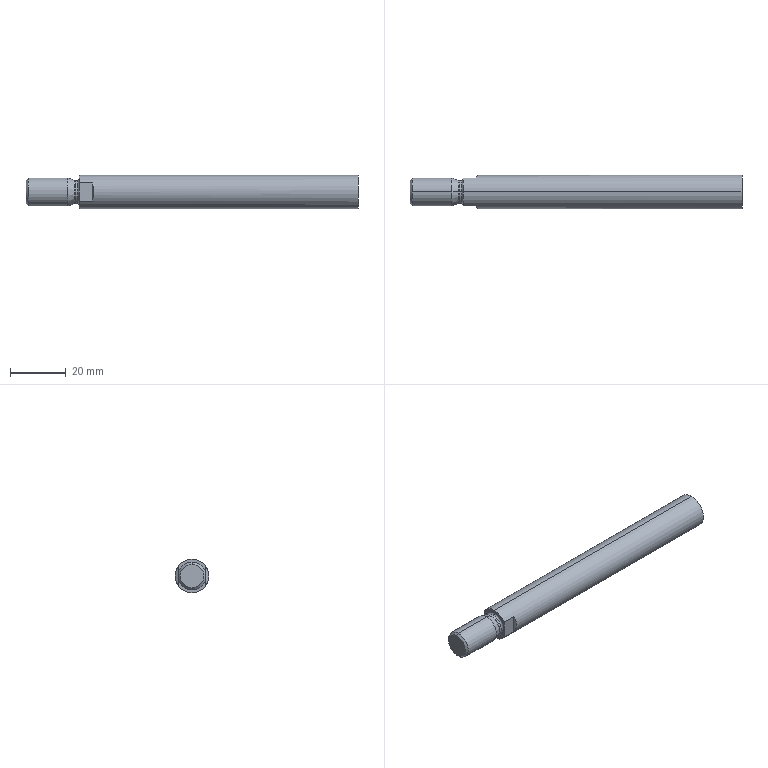Part | STEP file | Part 4 | 1 solid | 21 faces | box 119 x 12 x 12 mm | volume 12679 mm3 | plane 7 | cylinder 6 | torus 4 | cone 4 | commonest cylinder face diameters 8.2 x2 10 x2 12 x2
STEP:
#1=CARTESIAN_POINT('',(0.,0.,0.));
#2=DIRECTION('',(0.,0.,1.));
#3=DIRECTION('',(1.,0.,0.));
#4=AXIS2_PLACEMENT_3D('',#1,#2,#3);
#5=CARTESIAN_POINT('',(-7.699,0.,4.136));
#6=VERTEX_POINT('',#5);
#7=CARTESIAN_POINT('',(-7.494,0.,4.1));
#8=VERTEX_POINT('',#7);
#9=CARTESIAN_POINT('',(-7.494,0.,4.7));
#10=DIRECTION('',(0.,-1.,0.));
#11=DIRECTION('',(0.,0.,-1.));
#12=AXIS2_PLACEMENT_3D('',#9,#10,#11);
#13=CIRCLE('',#12,0.6);
#14=CARTESIAN_POINT('',(-7.494,0.,0.));
#15=DIRECTION('',(-1.,0.,0.));
#16=DIRECTION('',(0.,0.,1.));
#17=AXIS2_PLACEMENT_3D('',#14,#15,#16);
#18=TOROIDAL_SURFACE('',#17,4.7,0.6);
#19=CARTESIAN_POINT('',(6.283,-3.142));
#20=DIRECTION('',(0.,1.));
#21=VECTOR('',#20,1.);
#22=LINE('',#19,#21);
#23=(GEOMETRIC_REPRESENTATION_CONTEXT(2)PARAMETRIC_REPRESENTATION_CONTEXT()REPRESENTATION_CONTEXT('',''));
#24=DEFINITIONAL_REPRESENTATION('',(#22),#23);
#25=PCURVE('',#18,#24);
#26=CARTESIAN_POINT('',(-7.494,0.,0.));
#27=DIRECTION('',(-1.,0.,0.));
#28=DIRECTION('',(0.,0.,1.));
#29=AXIS2_PLACEMENT_3D('',#26,#27,#28);
#30=TOROIDAL_SURFACE('',#29,4.7,0.6);
#31=CARTESIAN_POINT('',(0.,-3.142));
#32=DIRECTION('',(0.,1.));
#33=VECTOR('',#32,1.);
#34=LINE('',#31,#33);
#35=(GEOMETRIC_REPRESENTATION_CONTEXT(2)PARAMETRIC_REPRESENTATION_CONTEXT()REPRESENTATION_CONTEXT('',''));
#36=DEFINITIONAL_REPRESENTATION('',(#34),#35);
#37=PCURVE('',#30,#36);
#38=SURFACE_CURVE('',#13,(#25,#37),.PCURVE_S1.);
#39=EDGE_CURVE('',#6,#8,#38,.T.);
#40=ORIENTED_EDGE('',*,*,#39,.T.);
#41=CARTESIAN_POINT('',(-7.494,0.,-4.1));
#42=VERTEX_POINT('',#41);
#43=CARTESIAN_POINT('',(-7.494,0.,0.));
#44=DIRECTION('',(1.,0.,0.));
#45=DIRECTION('',(0.,0.,1.));
#46=AXIS2_PLACEMENT_3D('',#43,#44,#45);
#47=CIRCLE('',#46,4.1);
#48=CARTESIAN_POINT('',(6.283,3.142));
#49=DIRECTION('',(-1.,0.));
#50=VECTOR('',#49,1.);
#51=LINE('',#48,#50);
#52=(GEOMETRIC_REPRESENTATION_CONTEXT(2)PARAMETRIC_REPRESENTATION_CONTEXT()REPRESENTATION_CONTEXT('',''));
#53=DEFINITIONAL_REPRESENTATION('',(#51),#52);
#54=PCURVE('',#18,#53);
#55=CARTESIAN_POINT('',(-7.6,0.,0.));
#56=DIRECTION('',(1.,0.,0.));
#57=DIRECTION('',(0.,0.,-1.));
#58=AXIS2_PLACEMENT_3D('',#55,#56,#57);
#59=CYLINDRICAL_SURFACE('',#58,4.1);
#60=CARTESIAN_POINT('',(3.142,0.1058));
#61=DIRECTION('',(1.,0.));
#62=VECTOR('',#61,1.);
#63=LINE('',#60,#62);
#64=(GEOMETRIC_REPRESENTATION_CONTEXT(2)PARAMETRIC_REPRESENTATION_CONTEXT()REPRESENTATION_CONTEXT('',''));
#65=DEFINITIONAL_REPRESENTATION('',(#63),#64);
#66=PCURVE('',#59,#65);
#67=SURFACE_CURVE('',#47,(#54,#66),.PCURVE_S1.);
#68=EDGE_CURVE('',#8,#42,#67,.T.);
#69=ORIENTED_EDGE('',*,*,#68,.T.);
#70=CARTESIAN_POINT('',(-7.699,0.,-4.136));
#71=VERTEX_POINT('',#70);
#72=CARTESIAN_POINT('',(-7.494,0.,-4.7));
#73=DIRECTION('',(0.,1.,0.));
#74=DIRECTION('',(0.,0.,1.));
#75=AXIS2_PLACEMENT_3D('',#72,#73,#74);
#76=CIRCLE('',#75,0.6);
#77=CARTESIAN_POINT('',(3.142,-3.142));
#78=DIRECTION('',(0.,1.));
#79=VECTOR('',#78,1.);
#80=LINE('',#77,#79);
#81=(GEOMETRIC_REPRESENTATION_CONTEXT(2)PARAMETRIC_REPRESENTATION_CONTEXT()REPRESENTATION_CONTEXT('',''));
#82=DEFINITIONAL_REPRESENTATION('',(#80),#81);
#83=PCURVE('',#18,#82);
#84=CARTESIAN_POINT('',(3.142,-3.142));
#85=DIRECTION('',(0.,1.));
#86=VECTOR('',#85,1.);
#87=LINE('',#84,#86);
#88=(GEOMETRIC_REPRESENTATION_CONTEXT(2)PARAMETRIC_REPRESENTATION_CONTEXT()REPRESENTATION_CONTEXT('',''));
#89=DEFINITIONAL_REPRESENTATION('',(#87),#88);
#90=PCURVE('',#30,#89);
#91=SURFACE_CURVE('',#76,(#83,#90),.PCURVE_S1.);
#92=EDGE_CURVE('',#71,#42,#91,.T.);
#93=ORIENTED_EDGE('',*,*,#92,.F.);
#94=CARTESIAN_POINT('',(-7.699,0.,0.));
#95=DIRECTION('',(-1.,0.,0.));
#96=DIRECTION('',(0.,0.,1.));
#97=AXIS2_PLACEMENT_3D('',#94,#95,#96);
#98=CIRCLE('',#97,4.136);
#99=CARTESIAN_POINT('',(0.,2.793));
#100=DIRECTION('',(1.,0.));
#101=VECTOR('',#100,1.);
#102=LINE('',#99,#101);
#103=(GEOMETRIC_REPRESENTATION_CONTEXT(2)PARAMETRIC_REPRESENTATION_CONTEXT()REPRESENTATION_CONTEXT('',''));
#104=DEFINITIONAL_REPRESENTATION('',(#102),#103);
#105=PCURVE('',#18,#104);
#106=CARTESIAN_POINT('',(-7.6,0.,0.));
#107=DIRECTION('',(-1.,0.,0.));
#108=DIRECTION('',(0.,0.,1.));
#109=AXIS2_PLACEMENT_3D('',#106,#107,#108);
#110=CONICAL_SURFACE('',#109,4.1,0.3491);
#111=CARTESIAN_POINT('',(0.,0.09942));
#112=DIRECTION('',(1.,0.));
#113=VECTOR('',#112,1.);
#114=LINE('',#111,#113);
#115=(GEOMETRIC_REPRESENTATION_CONTEXT(2)PARAMETRIC_REPRESENTATION_CONTEXT()REPRESENTATION_CONTEXT('',''));
#116=DEFINITIONAL_REPRESENTATION('',(#114),#115);
#117=PCURVE('',#110,#116);
#118=SURFACE_CURVE('',#98,(#105,#117),.PCURVE_S1.);
#119=EDGE_CURVE('',#71,#6,#118,.T.);
#120=ORIENTED_EDGE('',*,*,#119,.T.);
#121=EDGE_LOOP('',(#40,#69,#93,#120));
#122=FACE_BOUND('',#121,.F.);
#123=ADVANCED_FACE('',(#122),#18,.F.);
#124=CARTESIAN_POINT('',(-6.7,0.,4.1));
#125=VERTEX_POINT('',#124);
#126=CARTESIAN_POINT('',(-6.1,0.,4.7));
#127=VERTEX_POINT('',#126);
#128=CARTESIAN_POINT('',(-6.7,0.,4.7));
#129=DIRECTION('',(0.,-1.,0.));
#130=DIRECTION('',(0.,0.,-1.));
#131=AXIS2_PLACEMENT_3D('',#128,#129,#130);
#132=CIRCLE('',#131,0.6);
#133=CARTESIAN_POINT('',(-6.7,0.,0.));
#134=DIRECTION('',(-1.,0.,0.));
#135=DIRECTION('',(0.,0.,1.));
#136=AXIS2_PLACEMENT_3D('',#133,#134,#135);
#137=TOROIDAL_SURFACE('',#136,4.7,0.6);
#138=CARTESIAN_POINT('',(6.283,3.142));
#139=DIRECTION('',(0.,1.));
#140=VECTOR('',#139,1.);
#141=LINE('',#138,#140);
#142=(GEOMETRIC_REPRESENTATION_CONTEXT(2)PARAMETRIC_REPRESENTATION_CONTEXT()REPRESENTATION_CONTEXT('',''));
#143=DEFINITIONAL_REPRESENTATION('',(#141),#142);
#144=PCURVE('',#137,#143);
#145=CARTESIAN_POINT('',(-6.7,0.,0.));
#146=DIRECTION('',(-1.,0.,0.));
#147=DIRECTION('',(0.,0.,1.));
#148=AXIS2_PLACEMENT_3D('',#145,#146,#147);
#149=TOROIDAL_SURFACE('',#148,4.7,0.6);
#150=CARTESIAN_POINT('',(0.,3.142));
#151=DIRECTION('',(0.,1.));
#152=VECTOR('',#151,1.);
#153=LINE('',#150,#152);
#154=(GEOMETRIC_REPRESENTATION_CONTEXT(2)PARAMETRIC_REPRESENTATION_CONTEXT()REPRESENTATION_CONTEXT('',''));
#155=DEFINITIONAL_REPRESENTATION('',(#153),#154);
#156=PCURVE('',#149,#155);
#157=SURFACE_CURVE('',#132,(#144,#156),.PCURVE_S1.);
#158=EDGE_CURVE('',#125,#127,#157,.T.);
#159=ORIENTED_EDGE('',*,*,#158,.T.);
#160=CARTESIAN_POINT('',(-6.1,0.,-4.7));
#161=VERTEX_POINT('',#160);
#162=CARTESIAN_POINT('',(-6.1,0.,0.));
#163=DIRECTION('',(1.,0.,0.));
#164=DIRECTION('',(0.,0.,1.));
#165=AXIS2_PLACEMENT_3D('',#162,#163,#164);
#166=CIRCLE('',#165,4.7);
#167=CARTESIAN_POINT('',(6.283,4.712));
#168=DIRECTION('',(-1.,0.));
#169=VECTOR('',#168,1.);
#170=LINE('',#167,#169);
#171=(GEOMETRIC_REPRESENTATION_CONTEXT(2)PARAMETRIC_REPRESENTATION_CONTEXT()REPRESENTATION_CONTEXT('',''));
#172=DEFINITIONAL_REPRESENTATION('',(#170),#171);
#173=PCURVE('',#137,#172);
#174=CARTESIAN_POINT('',(-6.1,6.,0.));
#175=DIRECTION('',(-1.,0.,0.));
#176=DIRECTION('',(0.,0.,1.));
#177=AXIS2_PLACEMENT_3D('',#174,#175,#176);
#178=PLANE('',#177);
#179=CARTESIAN_POINT('',(4.7,-6.));
#180=CARTESIAN_POINT('',(4.7,-14.141));
#181=CARTESIAN_POINT('',(-2.35,-10.07));
#182=CARTESIAN_POINT('',(-9.4,-6.));
#183=CARTESIAN_POINT('',(-2.35,-1.93));
#184=CARTESIAN_POINT('',(4.7,2.141));
#185=CARTESIAN_POINT('',(4.7,-6.));
#186=(BOUNDED_CURVE()B_SPLINE_CURVE(2,(#179,#180,#181,#182,#183,#184,#185),.UNSPECIFIED.,.T.,.F.)B_SPLINE_CURVE_WITH_KNOTS((1,2,2,2,2,1),(-2.094,0.,2.094,4.189,6.283,8.378),.UNSPECIFIED.)CURVE()GEOMETRIC_REPRESENTATION_ITEM()RATIONAL_B_SPLINE_CURVE((1.,0.5,1.,0.5,1.,0.5,1.))REPRESENTATION_ITEM(''));
#187=(GEOMETRIC_REPRESENTATION_CONTEXT(2)PARAMETRIC_REPRESENTATION_CONTEXT()REPRESENTATION_CONTEXT('',''));
#188=DEFINITIONAL_REPRESENTATION('',(#186),#187);
#189=PCURVE('',#178,#188);
#190=SURFACE_CURVE('',#166,(#173,#189),.PCURVE_S1.);
#191=EDGE_CURVE('',#127,#161,#190,.T.);
#192=ORIENTED_EDGE('',*,*,#191,.T.);
#193=CARTESIAN_POINT('',(-6.7,0.,-4.1));
#194=VERTEX_POINT('',#193);
#195=CARTESIAN_POINT('',(-6.7,0.,-4.7));
#196=DIRECTION('',(0.,1.,0.));
#197=DIRECTION('',(0.,0.,1.));
#198=AXIS2_PLACEMENT_3D('',#195,#196,#197);
#199=CIRCLE('',#198,0.6);
#200=CARTESIAN_POINT('',(3.142,3.142));
#201=DIRECTION('',(0.,1.));
#202=VECTOR('',#201,1.);
#203=LINE('',#200,#202);
#204=(GEOMETRIC_REPRESENTATION_CONTEXT(2)PARAMETRIC_REPRESENTATION_CONTEXT()REPRESENTATION_CONTEXT('',''));
#205=DEFINITIONAL_REPRESENTATION('',(#203),#204);
#206=PCURVE('',#137,#205);
#207=CARTESIAN_POINT('',(3.142,3.142));
#208=DIRECTION('',(0.,1.));
#209=VECTOR('',#208,1.);
#210=LINE('',#207,#209);
#211=(GEOMETRIC_REPRESENTATION_CONTEXT(2)PARAMETRIC_REPRESENTATION_CONTEXT()REPRESENTATION_CONTEXT('',''));
#212=DEFINITIONAL_REPRESENTATION('',(#210),#211);
#213=PCURVE('',#149,#212);
#214=SURFACE_CURVE('',#199,(#206,#213),.PCURVE_S1.);
#215=EDGE_CURVE('',#194,#161,#214,.T.);
#216=ORIENTED_EDGE('',*,*,#215,.F.);
#217=CARTESIAN_POINT('',(-6.7,0.,0.));
#218=DIRECTION('',(-1.,0.,0.));
#219=DIRECTION('',(0.,0.,1.));
#220=AXIS2_PLACEMENT_3D('',#217,#218,#219);
#221=CIRCLE('',#220,4.1);
#222=CARTESIAN_POINT('',(0.,3.142));
#223=DIRECTION('',(1.,0.));
#224=VECTOR('',#223,1.);
#225=LINE('',#222,#224);
#226=(GEOMETRIC_REPRESENTATION_CONTEXT(2)PARAMETRIC_REPRESENTATION_CONTEXT()REPRESENTATION_CONTEXT('',''));
#227=DEFINITIONAL_REPRESENTATION('',(#225),#226);
#228=PCURVE('',#137,#227);
#229=CARTESIAN_POINT('',(9.425,0.9));
#230=DIRECTION('',(-1.,0.));
#231=VECTOR('',#230,1.);
#232=LINE('',#229,#231);
#233=(GEOMETRIC_REPRESENTATION_CONTEXT(2)PARAMETRIC_REPRESENTATION_CONTEXT()REPRESENTATION_CONTEXT('',''));
#234=DEFINITIONAL_REPRESENTATION('',(#232),#233);
#235=PCURVE('',#59,#234);
#236=SURFACE_CURVE('',#221,(#228,#235),.PCURVE_S1.);
#237=EDGE_CURVE('',#194,#125,#236,.T.);
#238=ORIENTED_EDGE('',*,*,#237,.T.);
#239=EDGE_LOOP('',(#159,#192,#216,#238));
#240=FACE_BOUND('',#239,.F.);
#241=ADVANCED_FACE('',(#240),#137,.F.);
#242=CARTESIAN_POINT('',(-25.1,0.,4.233));
#243=VERTEX_POINT('',#242);
#244=CARTESIAN_POINT('',(-25.1,0.,-4.233));
#245=VERTEX_POINT('',#244);
#246=CARTESIAN_POINT('',(-25.1,0.,0.));
#247=DIRECTION('',(-1.,0.,0.));
#248=DIRECTION('',(0.,0.,1.));
#249=AXIS2_PLACEMENT_3D('',#246,#247,#248);
#250=CIRCLE('',#249,4.233);
#251=CARTESIAN_POINT('',(-25.1,0.,0.));
#252=DIRECTION('',(1.,0.,0.));
#253=DIRECTION('',(0.,0.,-1.));
#254=AXIS2_PLACEMENT_3D('',#251,#252,#253);
#255=CONICAL_SURFACE('',#254,4.233,0.7854);
#256=CARTESIAN_POINT('',(3.142,0.));
#257=DIRECTION('',(-1.,0.));
#258=VECTOR('',#257,1.);
#259=LINE('',#256,#258);
#260=(GEOMETRIC_REPRESENTATION_CONTEXT(2)PARAMETRIC_REPRESENTATION_CONTEXT()REPRESENTATION_CONTEXT('',''));
#261=DEFINITIONAL_REPRESENTATION('',(#259),#260);
#262=PCURVE('',#255,#261);
#263=CARTESIAN_POINT('',(-25.1,0.,0.));
#264=DIRECTION('',(-1.,0.,0.));
#265=DIRECTION('',(0.,0.,1.));
#266=AXIS2_PLACEMENT_3D('',#263,#264,#265);
#267=PLANE('',#266);
#268=CARTESIAN_POINT('',(0.,0.));
#269=DIRECTION('',(1.,0.));
#270=AXIS2_PLACEMENT_2D('',#268,#269);
#271=CIRCLE('',#270,4.233);
#272=(GEOMETRIC_REPRESENTATION_CONTEXT(2)PARAMETRIC_REPRESENTATION_CONTEXT()REPRESENTATION_CONTEXT('',''));
#273=DEFINITIONAL_REPRESENTATION('',(#271),#272);
#274=PCURVE('',#267,#273);
#275=SURFACE_CURVE('',#250,(#262,#274),.PCURVE_S1.);
#276=EDGE_CURVE('',#243,#245,#275,.T.);
#277=ORIENTED_EDGE('',*,*,#276,.F.);
#278=CARTESIAN_POINT('',(-24.333,0.,5.));
#279=VERTEX_POINT('',#278);
#280=CARTESIAN_POINT('',(-25.1,0.,4.233));
#281=DIRECTION('',(0.7071,0.,0.7071));
#282=VECTOR('',#281,1.);
#283=LINE('',#280,#282);
#284=CARTESIAN_POINT('',(3.142,0.));
#285=DIRECTION('',(0.,1.));
#286=VECTOR('',#285,1.);
#287=LINE('',#284,#286);
#288=(GEOMETRIC_REPRESENTATION_CONTEXT(2)PARAMETRIC_REPRESENTATION_CONTEXT()REPRESENTATION_CONTEXT('',''));
#289=DEFINITIONAL_REPRESENTATION('',(#287),#288);
#290=PCURVE('',#255,#289);
#291=CARTESIAN_POINT('',(-25.1,0.,0.));
#292=DIRECTION('',(1.,0.,0.));
#293=DIRECTION('',(0.,0.,-1.));
#294=AXIS2_PLACEMENT_3D('',#291,#292,#293);
#295=CONICAL_SURFACE('',#294,4.233,0.7854);
#296=CARTESIAN_POINT('',(3.142,0.));
#297=DIRECTION('',(0.,1.));
#298=VECTOR('',#297,1.);
#299=LINE('',#296,#298);
#300=(GEOMETRIC_REPRESENTATION_CONTEXT(2)PARAMETRIC_REPRESENTATION_CONTEXT()REPRESENTATION_CONTEXT('',''));
#301=DEFINITIONAL_REPRESENTATION('',(#299),#300);
#302=PCURVE('',#295,#301);
#303=SURFACE_CURVE('',#283,(#290,#302),.PCURVE_S1.);
#304=EDGE_CURVE('',#243,#279,#303,.T.);
#305=ORIENTED_EDGE('',*,*,#304,.T.);
#306=CARTESIAN_POINT('',(-24.333,0.,-5.));
#307=VERTEX_POINT('',#306);
#308=CARTESIAN_POINT('',(-24.333,0.,0.));
#309=DIRECTION('',(1.,0.,0.));
#310=DIRECTION('',(0.,0.,1.));
#311=AXIS2_PLACEMENT_3D('',#308,#309,#310);
#312=CIRCLE('',#311,5.);
#313=CARTESIAN_POINT('',(-3.142,0.767));
#314=DIRECTION('',(1.,0.));
#315=VECTOR('',#314,1.);
#316=LINE('',#313,#315);
#317=(GEOMETRIC_REPRESENTATION_CONTEXT(2)PARAMETRIC_REPRESENTATION_CONTEXT()REPRESENTATION_CONTEXT('',''));
#318=DEFINITIONAL_REPRESENTATION('',(#316),#317);
#319=PCURVE('',#255,#318);
#320=CARTESIAN_POINT('',(-25.1,0.,0.));
#321=DIRECTION('',(1.,0.,0.));
#322=DIRECTION('',(0.,0.,-1.));
#323=AXIS2_PLACEMENT_3D('',#320,#321,#322);
#324=CYLINDRICAL_SURFACE('',#323,5.);
#325=CARTESIAN_POINT('',(-3.142,0.767));
#326=DIRECTION('',(1.,0.));
#327=VECTOR('',#326,1.);
#328=LINE('',#325,#327);
#329=(GEOMETRIC_REPRESENTATION_CONTEXT(2)PARAMETRIC_REPRESENTATION_CONTEXT()REPRESENTATION_CONTEXT('',''));
#330=DEFINITIONAL_REPRESENTATION('',(#328),#329);
#331=PCURVE('',#324,#330);
#332=SURFACE_CURVE('',#312,(#319,#331),.PCURVE_S1.);
#333=EDGE_CURVE('',#307,#279,#332,.T.);
#334=ORIENTED_EDGE('',*,*,#333,.F.);
#335=CARTESIAN_POINT('',(-25.1,0.,-4.233));
#336=DIRECTION('',(0.7071,0.,-0.7071));
#337=VECTOR('',#336,1.);
#338=LINE('',#335,#337);
#339=CARTESIAN_POINT('',(0.,0.));
#340=DIRECTION('',(0.,1.));
#341=VECTOR('',#340,1.);
#342=LINE('',#339,#341);
#343=(GEOMETRIC_REPRESENTATION_CONTEXT(2)PARAMETRIC_REPRESENTATION_CONTEXT()REPRESENTATION_CONTEXT('',''));
#344=DEFINITIONAL_REPRESENTATION('',(#342),#343);
#345=PCURVE('',#255,#344);
#346=CARTESIAN_POINT('',(6.283,0.));
#347=DIRECTION('',(0.,1.));
#348=VECTOR('',#347,1.);
#349=LINE('',#346,#348);
#350=(GEOMETRIC_REPRESENTATION_CONTEXT(2)PARAMETRIC_REPRESENTATION_CONTEXT()REPRESENTATION_CONTEXT('',''));
#351=DEFINITIONAL_REPRESENTATION('',(#349),#350);
#352=PCURVE('',#295,#351);
#353=SURFACE_CURVE('',#338,(#345,#352),.PCURVE_S1.);
#354=EDGE_CURVE('',#245,#307,#353,.T.);
#355=ORIENTED_EDGE('',*,*,#354,.F.);
#356=EDGE_LOOP('',(#277,#305,#334,#355));
#357=FACE_BOUND('',#356,.T.);
#358=ADVANCED_FACE('',(#357),#255,.T.);
#359=ORIENTED_EDGE('',*,*,#333,.T.);
#360=CARTESIAN_POINT('',(-10.073,0.,5.));
#361=VERTEX_POINT('',#360);
#362=CARTESIAN_POINT('',(-25.1,0.,5.));
#363=DIRECTION('',(1.,0.,0.));
#364=VECTOR('',#363,1.);
#365=LINE('',#362,#364);
#366=CARTESIAN_POINT('',(3.142,0.));
#367=DIRECTION('',(0.,1.));
#368=VECTOR('',#367,1.);
#369=LINE('',#366,#368);
#370=(GEOMETRIC_REPRESENTATION_CONTEXT(2)PARAMETRIC_REPRESENTATION_CONTEXT()REPRESENTATION_CONTEXT('',''));
#371=DEFINITIONAL_REPRESENTATION('',(#369),#370);
#372=PCURVE('',#324,#371);
#373=CARTESIAN_POINT('',(-25.1,0.,0.));
#374=DIRECTION('',(1.,0.,0.));
#375=DIRECTION('',(0.,0.,-1.));
#376=AXIS2_PLACEMENT_3D('',#373,#374,#375);
#377=CYLINDRICAL_SURFACE('',#376,5.);
#378=CARTESIAN_POINT('',(3.142,0.));
#379=DIRECTION('',(0.,1.));
#380=VECTOR('',#379,1.);
#381=LINE('',#378,#380);
#382=(GEOMETRIC_REPRESENTATION_CONTEXT(2)PARAMETRIC_REPRESENTATION_CONTEXT()REPRESENTATION_CONTEXT('',''));
#383=DEFINITIONAL_REPRESENTATION('',(#381),#382);
#384=PCURVE('',#377,#383);
#385=SURFACE_CURVE('',#365,(#372,#384),.PCURVE_S1.);
#386=EDGE_CURVE('',#279,#361,#385,.T.);
#387=ORIENTED_EDGE('',*,*,#386,.T.);
#388=CARTESIAN_POINT('',(-10.073,0.,-5.));
#389=VERTEX_POINT('',#388);
#390=CARTESIAN_POINT('',(-10.073,0.,0.));
#391=DIRECTION('',(-1.,0.,0.));
#392=DIRECTION('',(0.,0.,1.));
#393=AXIS2_PLACEMENT_3D('',#390,#391,#392);
#394=CIRCLE('',#393,5.);
#395=CARTESIAN_POINT('',(3.142,15.027));
#396=DIRECTION('',(-1.,0.));
#397=VECTOR('',#396,1.);
#398=LINE('',#395,#397);
#399=(GEOMETRIC_REPRESENTATION_CONTEXT(2)PARAMETRIC_REPRESENTATION_CONTEXT()REPRESENTATION_CONTEXT('',''));
#400=DEFINITIONAL_REPRESENTATION('',(#398),#399);
#401=PCURVE('',#324,#400);
#402=CARTESIAN_POINT('',(-7.6,0.,0.));
#403=DIRECTION('',(-1.,0.,0.));
#404=DIRECTION('',(0.,0.,1.));
#405=AXIS2_PLACEMENT_3D('',#402,#403,#404);
#406=CONICAL_SURFACE('',#405,4.1,0.3491);
#407=CARTESIAN_POINT('',(0.,2.473));
#408=DIRECTION('',(1.,0.));
#409=VECTOR('',#408,1.);
#410=LINE('',#407,#409);
#411=(GEOMETRIC_REPRESENTATION_CONTEXT(2)PARAMETRIC_REPRESENTATION_CONTEXT()REPRESENTATION_CONTEXT('',''));
#412=DEFINITIONAL_REPRESENTATION('',(#410),#411);
#413=PCURVE('',#406,#412);
#414=SURFACE_CURVE('',#394,(#401,#413),.PCURVE_S1.);
#415=EDGE_CURVE('',#361,#389,#414,.T.);
#416=ORIENTED_EDGE('',*,*,#415,.T.);
#417=CARTESIAN_POINT('',(-25.1,0.,-5.));
#418=DIRECTION('',(1.,0.,0.));
#419=VECTOR('',#418,1.);
#420=LINE('',#417,#419);
#421=CARTESIAN_POINT('',(0.,0.));
#422=DIRECTION('',(0.,1.));
#423=VECTOR('',#422,1.);
#424=LINE('',#421,#423);
#425=(GEOMETRIC_REPRESENTATION_CONTEXT(2)PARAMETRIC_REPRESENTATION_CONTEXT()REPRESENTATION_CONTEXT('',''));
#426=DEFINITIONAL_REPRESENTATION('',(#424),#425);
#427=PCURVE('',#324,#426);
#428=CARTESIAN_POINT('',(6.283,0.));
#429=DIRECTION('',(0.,1.));
#430=VECTOR('',#429,1.);
#431=LINE('',#428,#430);
#432=(GEOMETRIC_REPRESENTATION_CONTEXT(2)PARAMETRIC_REPRESENTATION_CONTEXT()REPRESENTATION_CONTEXT('',''));
#433=DEFINITIONAL_REPRESENTATION('',(#431),#432);
#434=PCURVE('',#377,#433);
#435=SURFACE_CURVE('',#420,(#427,#434),.PCURVE_S1.);
#436=EDGE_CURVE('',#307,#389,#435,.T.);
#437=ORIENTED_EDGE('',*,*,#436,.F.);
#438=EDGE_LOOP('',(#359,#387,#416,#437));
#439=FACE_BOUND('',#438,.T.);
#440=ADVANCED_FACE('',(#439),#324,.T.);
#441=CARTESIAN_POINT('',(-7.699,0.,0.));
#442=DIRECTION('',(-1.,0.,0.));
#443=DIRECTION('',(0.,0.,1.));
#444=AXIS2_PLACEMENT_3D('',#441,#442,#443);
#445=CIRCLE('',#444,4.136);
#446=CARTESIAN_POINT('',(0.,0.09942));
#447=DIRECTION('',(1.,0.));
#448=VECTOR('',#447,1.);
#449=LINE('',#446,#448);
#450=(GEOMETRIC_REPRESENTATION_CONTEXT(2)PARAMETRIC_REPRESENTATION_CONTEXT()REPRESENTATION_CONTEXT('',''));
#451=DEFINITIONAL_REPRESENTATION('',(#449),#450);
#452=PCURVE('',#406,#451);
#453=CARTESIAN_POINT('',(0.,2.793));
#454=DIRECTION('',(1.,0.));
#455=VECTOR('',#454,1.);
#456=LINE('',#453,#455);
#457=(GEOMETRIC_REPRESENTATION_CONTEXT(2)PARAMETRIC_REPRESENTATION_CONTEXT()REPRESENTATION_CONTEXT('',''));
#458=DEFINITIONAL_REPRESENTATION('',(#456),#457);
#459=PCURVE('',#30,#458);
#460=SURFACE_CURVE('',#445,(#452,#459),.PCURVE_S1.);
#461=EDGE_CURVE('',#6,#71,#460,.T.);
#462=ORIENTED_EDGE('',*,*,#461,.T.);
#463=CARTESIAN_POINT('',(-7.6,0.,-4.1));
#464=DIRECTION('',(-0.9397,0.,-0.342));
#465=VECTOR('',#464,1.);
#466=LINE('',#463,#465);
#467=CARTESIAN_POINT('',(3.142,0.));
#468=DIRECTION('',(0.,1.));
#469=VECTOR('',#468,1.);
#470=LINE('',#467,#469);
#471=(GEOMETRIC_REPRESENTATION_CONTEXT(2)PARAMETRIC_REPRESENTATION_CONTEXT()REPRESENTATION_CONTEXT('',''));
#472=DEFINITIONAL_REPRESENTATION('',(#470),#471);
#473=PCURVE('',#406,#472);
#474=CARTESIAN_POINT('',(3.142,0.));
#475=DIRECTION('',(0.,1.));
#476=VECTOR('',#475,1.);
#477=LINE('',#474,#476);
#478=(GEOMETRIC_REPRESENTATION_CONTEXT(2)PARAMETRIC_REPRESENTATION_CONTEXT()REPRESENTATION_CONTEXT('',''));
#479=DEFINITIONAL_REPRESENTATION('',(#477),#478);
#480=PCURVE('',#110,#479);
#481=SURFACE_CURVE('',#466,(#473,#480),.PCURVE_S1.);
#482=EDGE_CURVE('',#71,#389,#481,.T.);
#483=ORIENTED_EDGE('',*,*,#482,.T.);
#484=ORIENTED_EDGE('',*,*,#415,.F.);
#485=CARTESIAN_POINT('',(-7.6,0.,4.1));
#486=DIRECTION('',(-0.9397,0.,0.342));
#487=VECTOR('',#486,1.);
#488=LINE('',#485,#487);
#489=CARTESIAN_POINT('',(0.,0.));
#490=DIRECTION('',(0.,1.));
#491=VECTOR('',#490,1.);
#492=LINE('',#489,#491);
#493=(GEOMETRIC_REPRESENTATION_CONTEXT(2)PARAMETRIC_REPRESENTATION_CONTEXT()REPRESENTATION_CONTEXT('',''));
#494=DEFINITIONAL_REPRESENTATION('',(#492),#493);
#495=PCURVE('',#406,#494);
#496=CARTESIAN_POINT('',(6.283,0.));
#497=DIRECTION('',(0.,1.));
#498=VECTOR('',#497,1.);
#499=LINE('',#496,#498);
#500=(GEOMETRIC_REPRESENTATION_CONTEXT(2)PARAMETRIC_REPRESENTATION_CONTEXT()REPRESENTATION_CONTEXT('',''));
#501=DEFINITIONAL_REPRESENTATION('',(#499),#500);
#502=PCURVE('',#110,#501);
#503=SURFACE_CURVE('',#488,(#495,#502),.PCURVE_S1.);
#504=EDGE_CURVE('',#6,#361,#503,.T.);
#505=ORIENTED_EDGE('',*,*,#504,.F.);
#506=EDGE_LOOP('',(#462,#483,#484,#505));
#507=FACE_BOUND('',#506,.T.);
#508=ADVANCED_FACE('',(#507),#406,.T.);
#509=CARTESIAN_POINT('',(-7.494,0.,0.));
#510=DIRECTION('',(1.,0.,0.));
#511=DIRECTION('',(0.,0.,1.));
#512=AXIS2_PLACEMENT_3D('',#509,#510,#511);
#513=CIRCLE('',#512,4.1);
#514=CARTESIAN_POINT('',(-7.6,0.,0.));
#515=DIRECTION('',(1.,0.,0.));
#516=DIRECTION('',(0.,0.,-1.));
#517=AXIS2_PLACEMENT_3D('',#514,#515,#516);
#518=CYLINDRICAL_SURFACE('',#517,4.1);
#519=CARTESIAN_POINT('',(-3.142,0.1058));
#520=DIRECTION('',(1.,0.));
#521=VECTOR('',#520,1.);
#522=LINE('',#519,#521);
#523=(GEOMETRIC_REPRESENTATION_CONTEXT(2)PARAMETRIC_REPRESENTATION_CONTEXT()REPRESENTATION_CONTEXT('',''));
#524=DEFINITIONAL_REPRESENTATION('',(#522),#523);
#525=PCURVE('',#518,#524);
#526=CARTESIAN_POINT('',(6.283,3.142));
#527=DIRECTION('',(-1.,0.));
#528=VECTOR('',#527,1.);
#529=LINE('',#526,#528);
#530=(GEOMETRIC_REPRESENTATION_CONTEXT(2)PARAMETRIC_REPRESENTATION_CONTEXT()REPRESENTATION_CONTEXT('',''));
#531=DEFINITIONAL_REPRESENTATION('',(#529),#530);
#532=PCURVE('',#30,#531);
#533=SURFACE_CURVE('',#513,(#525,#532),.PCURVE_S1.);
#534=EDGE_CURVE('',#42,#8,#533,.T.);
#535=ORIENTED_EDGE('',*,*,#534,.T.);
#536=CARTESIAN_POINT('',(-7.6,0.,4.1));
#537=DIRECTION('',(1.,0.,0.));
#538=VECTOR('',#537,1.);
#539=LINE('',#536,#538);
#540=CARTESIAN_POINT('',(3.142,0.));
#541=DIRECTION('',(0.,1.));
#542=VECTOR('',#541,1.);
#543=LINE('',#540,#542);
#544=(GEOMETRIC_REPRESENTATION_CONTEXT(2)PARAMETRIC_REPRESENTATION_CONTEXT()REPRESENTATION_CONTEXT('',''));
#545=DEFINITIONAL_REPRESENTATION('',(#543),#544);
#546=PCURVE('',#518,#545);
#547=CARTESIAN_POINT('',(3.142,0.));
#548=DIRECTION('',(0.,1.));
#549=VECTOR('',#548,1.);
#550=LINE('',#547,#549);
#551=(GEOMETRIC_REPRESENTATION_CONTEXT(2)PARAMETRIC_REPRESENTATION_CONTEXT()REPRESENTATION_CONTEXT('',''));
#552=DEFINITIONAL_REPRESENTATION('',(#550),#551);
#553=PCURVE('',#59,#552);
#554=SURFACE_CURVE('',#539,(#546,#553),.PCURVE_S1.);
#555=EDGE_CURVE('',#8,#125,#554,.T.);
#556=ORIENTED_EDGE('',*,*,#555,.T.);
#557=CARTESIAN_POINT('',(-6.7,0.,0.));
#558=DIRECTION('',(-1.,0.,0.));
#559=DIRECTION('',(0.,0.,1.));
#560=AXIS2_PLACEMENT_3D('',#557,#558,#559);
#561=CIRCLE('',#560,4.1);
#562=CARTESIAN_POINT('',(3.142,0.9));
#563=DIRECTION('',(-1.,0.));
#564=VECTOR('',#563,1.);
#565=LINE('',#562,#564);
#566=(GEOMETRIC_REPRESENTATION_CONTEXT(2)PARAMETRIC_REPRESENTATION_CONTEXT()REPRESENTATION_CONTEXT('',''));
#567=DEFINITIONAL_REPRESENTATION('',(#565),#566);
#568=PCURVE('',#518,#567);
#569=CARTESIAN_POINT('',(0.,3.142));
#570=DIRECTION('',(1.,0.));
#571=VECTOR('',#570,1.);
#572=LINE('',#569,#571);
#573=(GEOMETRIC_REPRESENTATION_CONTEXT(2)PARAMETRIC_REPRESENTATION_CONTEXT()REPRESENTATION_CONTEXT('',''));
#574=DEFINITIONAL_REPRESENTATION('',(#572),#573);
#575=PCURVE('',#149,#574);
#576=SURFACE_CURVE('',#561,(#568,#575),.PCURVE_S1.);
#577=EDGE_CURVE('',#125,#194,#576,.T.);
#578=ORIENTED_EDGE('',*,*,#577,.T.);
#579=CARTESIAN_POINT('',(-7.6,0.,-4.1));
#580=DIRECTION('',(1.,0.,0.));
#581=VECTOR('',#580,1.);
#582=LINE('',#579,#581);
#583=CARTESIAN_POINT('',(0.,0.));
#584=DIRECTION('',(0.,1.));
#585=VECTOR('',#584,1.);
#586=LINE('',#583,#585);
#587=(GEOMETRIC_REPRESENTATION_CONTEXT(2)PARAMETRIC_REPRESENTATION_CONTEXT()REPRESENTATION_CONTEXT('',''));
#588=DEFINITIONAL_REPRESENTATION('',(#586),#587);
#589=PCURVE('',#518,#588);
#590=CARTESIAN_POINT('',(6.283,0.));
#591=DIRECTION('',(0.,1.));
#592=VECTOR('',#591,1.);
#593=LINE('',#590,#592);
#594=(GEOMETRIC_REPRESENTATION_CONTEXT(2)PARAMETRIC_REPRESENTATION_CONTEXT()REPRESENTATION_CONTEXT('',''));
#595=DEFINITIONAL_REPRESENTATION('',(#593),#594);
#596=PCURVE('',#59,#595);
#597=SURFACE_CURVE('',#582,(#589,#596),.PCURVE_S1.);
#598=EDGE_CURVE('',#42,#194,#597,.T.);
#599=ORIENTED_EDGE('',*,*,#598,.F.);
#600=EDGE_LOOP('',(#535,#556,#578,#599));
#601=FACE_BOUND('',#600,.T.);
#602=ADVANCED_FACE('',(#601),#518,.T.);
#603=CARTESIAN_POINT('',(-6.1,5.,3.317));
#604=VERTEX_POINT('',#603);
#605=CARTESIAN_POINT('',(-6.1,0.,6.));
#606=VERTEX_POINT('',#605);
#607=CARTESIAN_POINT('',(-6.1,0.,0.));
#608=DIRECTION('',(1.,0.,0.));
#609=DIRECTION('',(0.,0.,-1.));
#610=AXIS2_PLACEMENT_3D('',#607,#608,#609);
#611=CIRCLE('',#610,6.);
#612=CARTESIAN_POINT('',(-6.1,0.,0.));
#613=DIRECTION('',(1.,0.,0.));
#614=DIRECTION('',(0.,0.,-1.));
#615=AXIS2_PLACEMENT_3D('',#612,#613,#614);
#616=CYLINDRICAL_SURFACE('',#615,6.);
#617=CARTESIAN_POINT('',(0.,0.));
#618=DIRECTION('',(1.,0.));
#619=VECTOR('',#618,1.);
#620=LINE('',#617,#619);
#621=(GEOMETRIC_REPRESENTATION_CONTEXT(2)PARAMETRIC_REPRESENTATION_CONTEXT()REPRESENTATION_CONTEXT('',''));
#622=DEFINITIONAL_REPRESENTATION('',(#620),#621);
#623=PCURVE('',#616,#622);
#624=CARTESIAN_POINT('',(-6.,-6.));
#625=CARTESIAN_POINT('',(-6.,4.392));
#626=CARTESIAN_POINT('',(3.,-0.8038));
#627=CARTESIAN_POINT('',(12.,-6.));
#628=CARTESIAN_POINT('',(3.,-11.196));
#629=CARTESIAN_POINT('',(-6.,-16.392));
#630=CARTESIAN_POINT('',(-6.,-6.));
#631=(BOUNDED_CURVE()B_SPLINE_CURVE(2,(#624,#625,#626,#627,#628,#629,#630),.UNSPECIFIED.,.T.,.F.)B_SPLINE_CURVE_WITH_KNOTS((1,2,2,2,2,1),(-2.094,0.,2.094,4.189,6.283,8.378),.UNSPECIFIED.)CURVE()GEOMETRIC_REPRESENTATION_ITEM()RATIONAL_B_SPLINE_CURVE((1.,0.5,1.,0.5,1.,0.5,1.))REPRESENTATION_ITEM(''));
#632=(GEOMETRIC_REPRESENTATION_CONTEXT(2)PARAMETRIC_REPRESENTATION_CONTEXT()REPRESENTATION_CONTEXT('',''));
#633=DEFINITIONAL_REPRESENTATION('',(#631),#632);
#634=PCURVE('',#178,#633);
#635=SURFACE_CURVE('',#611,(#623,#634),.PCURVE_S1.);
#636=EDGE_CURVE('',#604,#606,#635,.T.);
#637=ORIENTED_EDGE('',*,*,#636,.T.);
#638=CARTESIAN_POINT('',(93.9,0.,6.));
#639=VERTEX_POINT('',#638);
#640=CARTESIAN_POINT('',(-6.1,0.,6.));
#641=DIRECTION('',(1.,0.,0.));
#642=VECTOR('',#641,1.);
#643=LINE('',#640,#642);
#644=CARTESIAN_POINT('',(3.142,0.));
#645=DIRECTION('',(0.,1.));
#646=VECTOR('',#645,1.);
#647=LINE('',#644,#646);
#648=(GEOMETRIC_REPRESENTATION_CONTEXT(2)PARAMETRIC_REPRESENTATION_CONTEXT()REPRESENTATION_CONTEXT('',''));
#649=DEFINITIONAL_REPRESENTATION('',(#647),#648);
#650=PCURVE('',#616,#649);
#651=CARTESIAN_POINT('',(-6.1,0.,0.));
#652=DIRECTION('',(1.,0.,0.));
#653=DIRECTION('',(0.,0.,-1.));
#654=AXIS2_PLACEMENT_3D('',#651,#652,#653);
#655=CYLINDRICAL_SURFACE('',#654,6.);
#656=CARTESIAN_POINT('',(3.142,0.));
#657=DIRECTION('',(0.,1.));
#658=VECTOR('',#657,1.);
#659=LINE('',#656,#658);
#660=(GEOMETRIC_REPRESENTATION_CONTEXT(2)PARAMETRIC_REPRESENTATION_CONTEXT()REPRESENTATION_CONTEXT('',''));
#661=DEFINITIONAL_REPRESENTATION('',(#659),#660);
#662=PCURVE('',#655,#661);
#663=SURFACE_CURVE('',#643,(#650,#662),.PCURVE_S1.);
#664=EDGE_CURVE('',#606,#639,#663,.T.);
#665=ORIENTED_EDGE('',*,*,#664,.T.);
#666=CARTESIAN_POINT('',(93.9,0.,-6.));
#667=VERTEX_POINT('',#666);
#668=CARTESIAN_POINT('',(93.9,0.,0.));
#669=DIRECTION('',(1.,0.,0.));
#670=DIRECTION('',(0.,0.,-1.));
#671=AXIS2_PLACEMENT_3D('',#668,#669,#670);
#672=CIRCLE('',#671,6.);
#673=CARTESIAN_POINT('',(0.,100.));
#674=DIRECTION('',(1.,0.));
#675=VECTOR('',#674,1.);
#676=LINE('',#673,#675);
#677=(GEOMETRIC_REPRESENTATION_CONTEXT(2)PARAMETRIC_REPRESENTATION_CONTEXT()REPRESENTATION_CONTEXT('',''));
#678=DEFINITIONAL_REPRESENTATION('',(#676),#677);
#679=PCURVE('',#616,#678);
#680=CARTESIAN_POINT('',(93.9,0.,0.));
#681=DIRECTION('',(1.,0.,0.));
#682=DIRECTION('',(0.,0.,-1.));
#683=AXIS2_PLACEMENT_3D('',#680,#681,#682);
#684=PLANE('',#683);
#685=CARTESIAN_POINT('',(0.,0.));
#686=DIRECTION('',(1.,0.));
#687=AXIS2_PLACEMENT_2D('',#685,#686);
#688=CIRCLE('',#687,6.);
#689=(GEOMETRIC_REPRESENTATION_CONTEXT(2)PARAMETRIC_REPRESENTATION_CONTEXT()REPRESENTATION_CONTEXT('',''));
#690=DEFINITIONAL_REPRESENTATION('',(#688),#689);
#691=PCURVE('',#684,#690);
#692=SURFACE_CURVE('',#672,(#679,#691),.PCURVE_S1.);
#693=EDGE_CURVE('',#667,#639,#692,.T.);
#694=ORIENTED_EDGE('',*,*,#693,.F.);
#695=CARTESIAN_POINT('',(-6.1,0.,-6.));
#696=VERTEX_POINT('',#695);
#697=CARTESIAN_POINT('',(-6.1,0.,-6.));
#698=DIRECTION('',(1.,0.,0.));
#699=VECTOR('',#698,1.);
#700=LINE('',#697,#699);
#701=CARTESIAN_POINT('',(0.,0.));
#702=DIRECTION('',(0.,1.));
#703=VECTOR('',#702,1.);
#704=LINE('',#701,#703);
#705=(GEOMETRIC_REPRESENTATION_CONTEXT(2)PARAMETRIC_REPRESENTATION_CONTEXT()REPRESENTATION_CONTEXT('',''));
#706=DEFINITIONAL_REPRESENTATION('',(#704),#705);
#707=PCURVE('',#616,#706);
#708=CARTESIAN_POINT('',(6.283,0.));
#709=DIRECTION('',(0.,1.));
#710=VECTOR('',#709,1.);
#711=LINE('',#708,#710);
#712=(GEOMETRIC_REPRESENTATION_CONTEXT(2)PARAMETRIC_REPRESENTATION_CONTEXT()REPRESENTATION_CONTEXT('',''));
#713=DEFINITIONAL_REPRESENTATION('',(#711),#712);
#714=PCURVE('',#655,#713);
#715=SURFACE_CURVE('',#700,(#707,#714),.PCURVE_S1.);
#716=EDGE_CURVE('',#696,#667,#715,.T.);
#717=ORIENTED_EDGE('',*,*,#716,.F.);
#718=CARTESIAN_POINT('',(-6.1,5.,-3.317));
#719=VERTEX_POINT('',#718);
#720=CARTESIAN_POINT('',(-6.1,0.,0.));
#721=DIRECTION('',(1.,0.,0.));
#722=DIRECTION('',(0.,0.,-1.));
#723=AXIS2_PLACEMENT_3D('',#720,#721,#722);
#724=CIRCLE('',#723,6.);
#725=CARTESIAN_POINT('',(0.,0.));
#726=DIRECTION('',(1.,0.));
#727=VECTOR('',#726,1.);
#728=LINE('',#725,#727);
#729=(GEOMETRIC_REPRESENTATION_CONTEXT(2)PARAMETRIC_REPRESENTATION_CONTEXT()REPRESENTATION_CONTEXT('',''));
#730=DEFINITIONAL_REPRESENTATION('',(#728),#729);
#731=PCURVE('',#616,#730);
#732=CARTESIAN_POINT('',(-6.,-6.));
#733=CARTESIAN_POINT('',(-6.,4.392));
#734=CARTESIAN_POINT('',(3.,-0.8038));
#735=CARTESIAN_POINT('',(12.,-6.));
#736=CARTESIAN_POINT('',(3.,-11.196));
#737=CARTESIAN_POINT('',(-6.,-16.392));
#738=CARTESIAN_POINT('',(-6.,-6.));
#739=(BOUNDED_CURVE()B_SPLINE_CURVE(2,(#732,#733,#734,#735,#736,#737,#738),.UNSPECIFIED.,.T.,.F.)B_SPLINE_CURVE_WITH_KNOTS((1,2,2,2,2,1),(-2.094,0.,2.094,4.189,6.283,8.378),.UNSPECIFIED.)CURVE()GEOMETRIC_REPRESENTATION_ITEM()RATIONAL_B_SPLINE_CURVE((1.,0.5,1.,0.5,1.,0.5,1.))REPRESENTATION_ITEM(''));
#740=(GEOMETRIC_REPRESENTATION_CONTEXT(2)PARAMETRIC_REPRESENTATION_CONTEXT()REPRESENTATION_CONTEXT('',''));
#741=DEFINITIONAL_REPRESENTATION('',(#739),#740);
#742=PCURVE('',#178,#741);
#743=SURFACE_CURVE('',#724,(#731,#742),.PCURVE_S1.);
#744=EDGE_CURVE('',#696,#719,#743,.T.);
#745=ORIENTED_EDGE('',*,*,#744,.T.);
#746=CARTESIAN_POINT('',(-1.4,5.,-3.317));
#747=VERTEX_POINT('',#746);
#748=CARTESIAN_POINT('',(-1.4,5.,-3.317));
#749=DIRECTION('',(-1.,0.,0.));
#750=VECTOR('',#749,1.);
#751=LINE('',#748,#750);
#752=CARTESIAN_POINT('',(0.9851,4.7));
#753=DIRECTION('',(0.,-1.));
#754=VECTOR('',#753,1.);
#755=LINE('',#752,#754);
#756=(GEOMETRIC_REPRESENTATION_CONTEXT(2)PARAMETRIC_REPRESENTATION_CONTEXT()REPRESENTATION_CONTEXT('',''));
#757=DEFINITIONAL_REPRESENTATION('',(#755),#756);
#758=PCURVE('',#616,#757);
#759=CARTESIAN_POINT('',(-1.4,5.,-3.317));
#760=DIRECTION('',(0.,-1.,0.));
#761=DIRECTION('',(0.,0.,-1.));
#762=AXIS2_PLACEMENT_3D('',#759,#760,#761);
#763=PLANE('',#762);
#764=CARTESIAN_POINT('',(0.,0.));
#765=DIRECTION('',(0.,-1.));
#766=VECTOR('',#765,1.);
#767=LINE('',#764,#766);
#768=(GEOMETRIC_REPRESENTATION_CONTEXT(2)PARAMETRIC_REPRESENTATION_CONTEXT()REPRESENTATION_CONTEXT('',''));
#769=DEFINITIONAL_REPRESENTATION('',(#767),#768);
#770=PCURVE('',#763,#769);
#771=SURFACE_CURVE('',#751,(#758,#770),.PCURVE_S1.);
#772=EDGE_CURVE('',#747,#719,#771,.T.);
#773=ORIENTED_EDGE('',*,*,#772,.F.);
#774=CARTESIAN_POINT('',(-1.4,5.,3.317));
#775=VERTEX_POINT('',#774);
#776=CARTESIAN_POINT('',(-1.4,5.,3.317));
#777=CARTESIAN_POINT('',(-0.6061,6.375,1.244));
#778=CARTESIAN_POINT('',(-0.6061,6.375,-1.244));
#779=CARTESIAN_POINT('',(-1.4,5.,-3.317));
#780=(BOUNDED_CURVE()B_SPLINE_CURVE(3,(#776,#777,#778,#779),.UNSPECIFIED.,.F.,.F.)B_SPLINE_CURVE_WITH_KNOTS((4,4),(5.697,6.869),.PIECEWISE_BEZIER_KNOTS.)CURVE()GEOMETRIC_REPRESENTATION_ITEM()RATIONAL_B_SPLINE_CURVE((1.,0.8889,0.8889,1.))REPRESENTATION_ITEM(''));
#781=CARTESIAN_POINT('',(2.156,4.7));
#782=CARTESIAN_POINT('',(2.14,4.732));
#783=CARTESIAN_POINT('',(2.106,4.794));
#784=CARTESIAN_POINT('',(2.055,4.881));
#785=CARTESIAN_POINT('',(2.003,4.961));
#786=CARTESIAN_POINT('',(1.95,5.033));
#787=CARTESIAN_POINT('',(1.897,5.096));
#788=CARTESIAN_POINT('',(1.843,5.151));
#789=CARTESIAN_POINT('',(1.789,5.197));
#790=CARTESIAN_POINT('',(1.735,5.232));
#791=CARTESIAN_POINT('',(1.68,5.258));
#792=CARTESIAN_POINT('',(1.626,5.274));
#793=CARTESIAN_POINT('',(1.571,5.279));
#794=CARTESIAN_POINT('',(1.516,5.274));
#795=CARTESIAN_POINT('',(1.461,5.258));
#796=CARTESIAN_POINT('',(1.407,5.232));
#797=CARTESIAN_POINT('',(1.352,5.197));
#798=CARTESIAN_POINT('',(1.298,5.151));
#799=CARTESIAN_POINT('',(1.245,5.096));
#800=CARTESIAN_POINT('',(1.192,5.033));
#801=CARTESIAN_POINT('',(1.139,4.961));
#802=CARTESIAN_POINT('',(1.087,4.881));
#803=CARTESIAN_POINT('',(1.036,4.794));
#804=CARTESIAN_POINT('',(1.002,4.732));
#805=CARTESIAN_POINT('',(0.9851,4.7));
#806=B_SPLINE_CURVE_WITH_KNOTS('',3,(#781,#782,#783,#784,#785,#786,#787,#788,#789,#790,#791,#792,#793,#794,#795,#796,#797,#798,#799,#800,#801,#802,#803,#804,#805),.UNSPECIFIED.,.F.,.F.,(4,1,1,1,1,1,1,1,1,1,1,1,1,1,1,1,1,1,1,1,1,1,4),(5.697,5.751,5.804,5.857,5.91,5.964,6.017,6.07,6.123,6.177,6.23,6.283,6.336,6.39,6.443,6.496,6.549,6.603,6.656,6.709,6.762,6.816,6.869),.QUASI_UNIFORM_KNOTS.);
#807=(GEOMETRIC_REPRESENTATION_CONTEXT(2)PARAMETRIC_REPRESENTATION_CONTEXT()REPRESENTATION_CONTEXT('',''));
#808=DEFINITIONAL_REPRESENTATION('',(#806),#807);
#809=PCURVE('',#616,#808);
#810=CARTESIAN_POINT('',(-1.4,5.,-3.317));
#811=DIRECTION('',(-0.866,0.5,0.));
#812=DIRECTION('',(-0.5,-0.866,0.));
#813=AXIS2_PLACEMENT_3D('',#810,#811,#812);
#814=PLANE('',#813);
#815=CARTESIAN_POINT('',(0.,6.633));
#816=CARTESIAN_POINT('',(-1.588,4.56));
#817=CARTESIAN_POINT('',(-1.588,2.073));
#818=CARTESIAN_POINT('',(0.,0.));
#819=(BOUNDED_CURVE()B_SPLINE_CURVE(3,(#815,#816,#817,#818),.UNSPECIFIED.,.F.,.F.)B_SPLINE_CURVE_WITH_KNOTS((4,4),(5.697,6.869),.PIECEWISE_BEZIER_KNOTS.)CURVE()GEOMETRIC_REPRESENTATION_ITEM()RATIONAL_B_SPLINE_CURVE((1.,0.8889,0.8889,1.))REPRESENTATION_ITEM(''));
#820=(GEOMETRIC_REPRESENTATION_CONTEXT(2)PARAMETRIC_REPRESENTATION_CONTEXT()REPRESENTATION_CONTEXT('',''));
#821=DEFINITIONAL_REPRESENTATION('',(#819),#820);
#822=PCURVE('',#814,#821);
#823=SURFACE_CURVE('',#780,(#809,#822),.PCURVE_S1.);
#824=EDGE_CURVE('',#775,#747,#823,.T.);
#825=ORIENTED_EDGE('',*,*,#824,.F.);
#826=CARTESIAN_POINT('',(-1.4,5.,3.317));
#827=DIRECTION('',(-1.,0.,0.));
#828=VECTOR('',#827,1.);
#829=LINE('',#826,#828);
#830=CARTESIAN_POINT('',(2.156,4.7));
#831=DIRECTION('',(0.,-1.));
#832=VECTOR('',#831,1.);
#833=LINE('',#830,#832);
#834=(GEOMETRIC_REPRESENTATION_CONTEXT(2)PARAMETRIC_REPRESENTATION_CONTEXT()REPRESENTATION_CONTEXT('',''));
#835=DEFINITIONAL_REPRESENTATION('',(#833),#834);
#836=PCURVE('',#616,#835);
#837=CARTESIAN_POINT('',(-6.633,0.));
#838=DIRECTION('',(0.,-1.));
#839=VECTOR('',#838,1.);
#840=LINE('',#837,#839);
#841=(GEOMETRIC_REPRESENTATION_CONTEXT(2)PARAMETRIC_REPRESENTATION_CONTEXT()REPRESENTATION_CONTEXT('',''));
#842=DEFINITIONAL_REPRESENTATION('',(#840),#841);
#843=PCURVE('',#763,#842);
#844=SURFACE_CURVE('',#829,(#836,#843),.PCURVE_S1.);
#845=EDGE_CURVE('',#775,#604,#844,.T.);
#846=ORIENTED_EDGE('',*,*,#845,.T.);
#847=EDGE_LOOP('',(#637,#665,#694,#717,#745,#773,#825,#846));
#848=FACE_BOUND('',#847,.T.);
#849=ADVANCED_FACE('',(#848),#616,.T.);
#850=ORIENTED_EDGE('',*,*,#664,.F.);
#851=CARTESIAN_POINT('',(-6.1,-5.,3.317));
#852=VERTEX_POINT('',#851);
#853=CARTESIAN_POINT('',(-6.1,0.,0.));
#854=DIRECTION('',(1.,0.,0.));
#855=DIRECTION('',(0.,0.,-1.));
#856=AXIS2_PLACEMENT_3D('',#853,#854,#855);
#857=CIRCLE('',#856,6.);
#858=CARTESIAN_POINT('',(0.,0.));
#859=DIRECTION('',(1.,0.));
#860=VECTOR('',#859,1.);
#861=LINE('',#858,#860);
#862=(GEOMETRIC_REPRESENTATION_CONTEXT(2)PARAMETRIC_REPRESENTATION_CONTEXT()REPRESENTATION_CONTEXT('',''));
#863=DEFINITIONAL_REPRESENTATION('',(#861),#862);
#864=PCURVE('',#655,#863);
#865=CARTESIAN_POINT('',(-6.,-6.));
#866=CARTESIAN_POINT('',(-6.,4.392));
#867=CARTESIAN_POINT('',(3.,-0.8038));
#868=CARTESIAN_POINT('',(12.,-6.));
#869=CARTESIAN_POINT('',(3.,-11.196));
#870=CARTESIAN_POINT('',(-6.,-16.392));
#871=CARTESIAN_POINT('',(-6.,-6.));
#872=(BOUNDED_CURVE()B_SPLINE_CURVE(2,(#865,#866,#867,#868,#869,#870,#871),.UNSPECIFIED.,.T.,.F.)B_SPLINE_CURVE_WITH_KNOTS((1,2,2,2,2,1),(-2.094,0.,2.094,4.189,6.283,8.378),.UNSPECIFIED.)CURVE()GEOMETRIC_REPRESENTATION_ITEM()RATIONAL_B_SPLINE_CURVE((1.,0.5,1.,0.5,1.,0.5,1.))REPRESENTATION_ITEM(''));
#873=(GEOMETRIC_REPRESENTATION_CONTEXT(2)PARAMETRIC_REPRESENTATION_CONTEXT()REPRESENTATION_CONTEXT('',''));
#874=DEFINITIONAL_REPRESENTATION('',(#872),#873);
#875=PCURVE('',#178,#874);
#876=SURFACE_CURVE('',#857,(#864,#875),.PCURVE_S1.);
#877=EDGE_CURVE('',#606,#852,#876,.T.);
#878=ORIENTED_EDGE('',*,*,#877,.T.);
#879=CARTESIAN_POINT('',(-1.4,-5.,3.317));
#880=VERTEX_POINT('',#879);
#881=CARTESIAN_POINT('',(-1.4,-5.,3.317));
#882=DIRECTION('',(-1.,0.,0.));
#883=VECTOR('',#882,1.);
#884=LINE('',#881,#883);
#885=CARTESIAN_POINT('',(4.127,4.7));
#886=DIRECTION('',(0.,-1.));
#887=VECTOR('',#886,1.);
#888=LINE('',#885,#887);
#889=(GEOMETRIC_REPRESENTATION_CONTEXT(2)PARAMETRIC_REPRESENTATION_CONTEXT()REPRESENTATION_CONTEXT('',''));
#890=DEFINITIONAL_REPRESENTATION('',(#888),#889);
#891=PCURVE('',#655,#890);
#892=CARTESIAN_POINT('',(-1.4,-5.,3.317));
#893=DIRECTION('',(0.,1.,0.));
#894=DIRECTION('',(0.,0.,1.));
#895=AXIS2_PLACEMENT_3D('',#892,#893,#894);
#896=PLANE('',#895);
#897=CARTESIAN_POINT('',(0.,0.));
#898=DIRECTION('',(0.,-1.));
#899=VECTOR('',#898,1.);
#900=LINE('',#897,#899);
#901=(GEOMETRIC_REPRESENTATION_CONTEXT(2)PARAMETRIC_REPRESENTATION_CONTEXT()REPRESENTATION_CONTEXT('',''));
#902=DEFINITIONAL_REPRESENTATION('',(#900),#901);
#903=PCURVE('',#896,#902);
#904=SURFACE_CURVE('',#884,(#891,#903),.PCURVE_S1.);
#905=EDGE_CURVE('',#880,#852,#904,.T.);
#906=ORIENTED_EDGE('',*,*,#905,.F.);
#907=CARTESIAN_POINT('',(-1.4,-5.,-3.317));
#908=VERTEX_POINT('',#907);
#909=CARTESIAN_POINT('',(-1.4,-5.,-3.317));
#910=CARTESIAN_POINT('',(-0.6061,-6.375,-1.244));
#911=CARTESIAN_POINT('',(-0.6061,-6.375,1.244));
#912=CARTESIAN_POINT('',(-1.4,-5.,3.317));
#913=(BOUNDED_CURVE()B_SPLINE_CURVE(3,(#909,#910,#911,#912),.UNSPECIFIED.,.F.,.F.)B_SPLINE_CURVE_WITH_KNOTS((4,4),(5.697,6.869),.PIECEWISE_BEZIER_KNOTS.)CURVE()GEOMETRIC_REPRESENTATION_ITEM()RATIONAL_B_SPLINE_CURVE((1.,0.8889,0.8889,1.))REPRESENTATION_ITEM(''));
#914=CARTESIAN_POINT('',(5.298,4.7));
#915=CARTESIAN_POINT('',(5.281,4.732));
#916=CARTESIAN_POINT('',(5.248,4.794));
#917=CARTESIAN_POINT('',(5.196,4.881));
#918=CARTESIAN_POINT('',(5.144,4.961));
#919=CARTESIAN_POINT('',(5.092,5.033));
#920=CARTESIAN_POINT('',(5.038,5.096));
#921=CARTESIAN_POINT('',(4.985,5.151));
#922=CARTESIAN_POINT('',(4.931,5.197));
#923=CARTESIAN_POINT('',(4.877,5.232));
#924=CARTESIAN_POINT('',(4.822,5.258));
#925=CARTESIAN_POINT('',(4.767,5.274));
#926=CARTESIAN_POINT('',(4.712,5.279));
#927=CARTESIAN_POINT('',(4.658,5.274));
#928=CARTESIAN_POINT('',(4.603,5.258));
#929=CARTESIAN_POINT('',(4.548,5.232));
#930=CARTESIAN_POINT('',(4.494,5.197));
#931=CARTESIAN_POINT('',(4.44,5.151));
#932=CARTESIAN_POINT('',(4.386,5.096));
#933=CARTESIAN_POINT('',(4.333,5.033));
#934=CARTESIAN_POINT('',(4.281,4.961));
#935=CARTESIAN_POINT('',(4.229,4.881));
#936=CARTESIAN_POINT('',(4.177,4.794));
#937=CARTESIAN_POINT('',(4.143,4.732));
#938=CARTESIAN_POINT('',(4.127,4.7));
#939=B_SPLINE_CURVE_WITH_KNOTS('',3,(#914,#915,#916,#917,#918,#919,#920,#921,#922,#923,#924,#925,#926,#927,#928,#929,#930,#931,#932,#933,#934,#935,#936,#937,#938),.UNSPECIFIED.,.F.,.F.,(4,1,1,1,1,1,1,1,1,1,1,1,1,1,1,1,1,1,1,1,1,1,4),(5.697,5.751,5.804,5.857,5.91,5.964,6.017,6.07,6.123,6.177,6.23,6.283,6.336,6.39,6.443,6.496,6.549,6.603,6.656,6.709,6.762,6.816,6.869),.QUASI_UNIFORM_KNOTS.);
#940=(GEOMETRIC_REPRESENTATION_CONTEXT(2)PARAMETRIC_REPRESENTATION_CONTEXT()REPRESENTATION_CONTEXT('',''));
#941=DEFINITIONAL_REPRESENTATION('',(#939),#940);
#942=PCURVE('',#655,#941);
#943=CARTESIAN_POINT('',(-1.4,-5.,3.317));
#944=DIRECTION('',(-0.866,-0.5,0.));
#945=DIRECTION('',(0.5,-0.866,0.));
#946=AXIS2_PLACEMENT_3D('',#943,#944,#945);
#947=PLANE('',#946);
#948=CARTESIAN_POINT('',(0.,-6.633));
#949=CARTESIAN_POINT('',(1.588,-4.56));
#950=CARTESIAN_POINT('',(1.588,-2.073));
#951=CARTESIAN_POINT('',(0.,0.));
#952=(BOUNDED_CURVE()B_SPLINE_CURVE(3,(#948,#949,#950,#951),.UNSPECIFIED.,.F.,.F.)B_SPLINE_CURVE_WITH_KNOTS((4,4),(5.697,6.869),.PIECEWISE_BEZIER_KNOTS.)CURVE()GEOMETRIC_REPRESENTATION_ITEM()RATIONAL_B_SPLINE_CURVE((1.,0.8889,0.8889,1.))REPRESENTATION_ITEM(''));
#953=(GEOMETRIC_REPRESENTATION_CONTEXT(2)PARAMETRIC_REPRESENTATION_CONTEXT()REPRESENTATION_CONTEXT('',''));
#954=DEFINITIONAL_REPRESENTATION('',(#952),#953);
#955=PCURVE('',#947,#954);
#956=SURFACE_CURVE('',#913,(#942,#955),.PCURVE_S1.);
#957=EDGE_CURVE('',#908,#880,#956,.T.);
#958=ORIENTED_EDGE('',*,*,#957,.F.);
#959=CARTESIAN_POINT('',(-6.1,-5.,-3.317));
#960=VERTEX_POINT('',#959);
#961=CARTESIAN_POINT('',(-1.4,-5.,-3.317));
#962=DIRECTION('',(-1.,0.,0.));
#963=VECTOR('',#962,1.);
#964=LINE('',#961,#963);
#965=CARTESIAN_POINT('',(5.298,4.7));
#966=DIRECTION('',(0.,-1.));
#967=VECTOR('',#966,1.);
#968=LINE('',#965,#967);
#969=(GEOMETRIC_REPRESENTATION_CONTEXT(2)PARAMETRIC_REPRESENTATION_CONTEXT()REPRESENTATION_CONTEXT('',''));
#970=DEFINITIONAL_REPRESENTATION('',(#968),#969);
#971=PCURVE('',#655,#970);
#972=CARTESIAN_POINT('',(-6.633,0.));
#973=DIRECTION('',(0.,-1.));
#974=VECTOR('',#973,1.);
#975=LINE('',#972,#974);
#976=(GEOMETRIC_REPRESENTATION_CONTEXT(2)PARAMETRIC_REPRESENTATION_CONTEXT()REPRESENTATION_CONTEXT('',''));
#977=DEFINITIONAL_REPRESENTATION('',(#975),#976);
#978=PCURVE('',#896,#977);
#979=SURFACE_CURVE('',#964,(#971,#978),.PCURVE_S1.);
#980=EDGE_CURVE('',#908,#960,#979,.T.);
#981=ORIENTED_EDGE('',*,*,#980,.T.);
#982=CARTESIAN_POINT('',(-6.1,0.,0.));
#983=DIRECTION('',(1.,0.,0.));
#984=DIRECTION('',(0.,0.,-1.));
#985=AXIS2_PLACEMENT_3D('',#982,#983,#984);
#986=CIRCLE('',#985,6.);
#987=CARTESIAN_POINT('',(0.,0.));
#988=DIRECTION('',(1.,0.));
#989=VECTOR('',#988,1.);
#990=LINE('',#987,#989);
#991=(GEOMETRIC_REPRESENTATION_CONTEXT(2)PARAMETRIC_REPRESENTATION_CONTEXT()REPRESENTATION_CONTEXT('',''));
#992=DEFINITIONAL_REPRESENTATION('',(#990),#991);
#993=PCURVE('',#655,#992);
#994=CARTESIAN_POINT('',(-6.,-6.));
#995=CARTESIAN_POINT('',(-6.,4.392));
#996=CARTESIAN_POINT('',(3.,-0.8038));
#997=CARTESIAN_POINT('',(12.,-6.));
#998=CARTESIAN_POINT('',(3.,-11.196));
#999=CARTESIAN_POINT('',(-6.,-16.392));
#1000=CARTESIAN_POINT('',(-6.,-6.));
#1001=(BOUNDED_CURVE()B_SPLINE_CURVE(2,(#994,#995,#996,#997,#998,#999,#1000),.UNSPECIFIED.,.T.,.F.)B_SPLINE_CURVE_WITH_KNOTS((1,2,2,2,2,1),(-2.094,0.,2.094,4.189,6.283,8.378),.UNSPECIFIED.)CURVE()GEOMETRIC_REPRESENTATION_ITEM()RATIONAL_B_SPLINE_CURVE((1.,0.5,1.,0.5,1.,0.5,1.))REPRESENTATION_ITEM(''));
#1002=(GEOMETRIC_REPRESENTATION_CONTEXT(2)PARAMETRIC_REPRESENTATION_CONTEXT()REPRESENTATION_CONTEXT('',''));
#1003=DEFINITIONAL_REPRESENTATION('',(#1001),#1002);
#1004=PCURVE('',#178,#1003);
#1005=SURFACE_CURVE('',#986,(#993,#1004),.PCURVE_S1.);
#1006=EDGE_CURVE('',#960,#696,#1005,.T.);
#1007=ORIENTED_EDGE('',*,*,#1006,.T.);
#1008=ORIENTED_EDGE('',*,*,#716,.T.);
#1009=CARTESIAN_POINT('',(93.9,0.,0.));
#1010=DIRECTION('',(1.,0.,0.));
#1011=DIRECTION('',(0.,0.,-1.));
#1012=AXIS2_PLACEMENT_3D('',#1009,#1010,#1011);
#1013=CIRCLE('',#1012,6.);
#1014=CARTESIAN_POINT('',(0.,100.));
#1015=DIRECTION('',(1.,0.));
#1016=VECTOR('',#1015,1.);
#1017=LINE('',#1014,#1016);
#1018=(GEOMETRIC_REPRESENTATION_CONTEXT(2)PARAMETRIC_REPRESENTATION_CONTEXT()REPRESENTATION_CONTEXT('',''));
#1019=DEFINITIONAL_REPRESENTATION('',(#1017),#1018);
#1020=PCURVE('',#655,#1019);
#1021=CARTESIAN_POINT('',(0.,0.));
#1022=DIRECTION('',(1.,0.));
#1023=AXIS2_PLACEMENT_2D('',#1021,#1022);
#1024=CIRCLE('',#1023,6.);
#1025=(GEOMETRIC_REPRESENTATION_CONTEXT(2)PARAMETRIC_REPRESENTATION_CONTEXT()REPRESENTATION_CONTEXT('',''));
#1026=DEFINITIONAL_REPRESENTATION('',(#1024),#1025);
#1027=PCURVE('',#684,#1026);
#1028=SURFACE_CURVE('',#1013,(#1020,#1027),.PCURVE_S1.);
#1029=EDGE_CURVE('',#639,#667,#1028,.T.);
#1030=ORIENTED_EDGE('',*,*,#1029,.F.);
#1031=EDGE_LOOP('',(#850,#878,#906,#958,#981,#1007,#1008,#1030));
#1032=FACE_BOUND('',#1031,.T.);
#1033=ADVANCED_FACE('',(#1032),#655,.T.);
#1034=ORIENTED_EDGE('',*,*,#191,.T.);
#1035=CARTESIAN_POINT('',(-6.1,0.,0.));
#1036=DIRECTION('',(1.,0.,0.));
#1037=DIRECTION('',(0.,0.,1.));
#1038=AXIS2_PLACEMENT_3D('',#1035,#1036,#1037);
#1039=CIRCLE('',#1038,4.7);
#1040=CARTESIAN_POINT('',(4.7,-6.));
#1041=CARTESIAN_POINT('',(4.7,-14.141));
#1042=CARTESIAN_POINT('',(-2.35,-10.07));
#1043=CARTESIAN_POINT('',(-9.4,-6.));
#1044=CARTESIAN_POINT('',(-2.35,-1.93));
#1045=CARTESIAN_POINT('',(4.7,2.141));
#1046=CARTESIAN_POINT('',(4.7,-6.));
#1047=(BOUNDED_CURVE()B_SPLINE_CURVE(2,(#1040,#1041,#1042,#1043,#1044,#1045,#1046),.UNSPECIFIED.,.T.,.F.)B_SPLINE_CURVE_WITH_KNOTS((1,2,2,2,2,1),(-2.094,0.,2.094,4.189,6.283,8.378),.UNSPECIFIED.)CURVE()GEOMETRIC_REPRESENTATION_ITEM()RATIONAL_B_SPLINE_CURVE((1.,0.5,1.,0.5,1.,0.5,1.))REPRESENTATION_ITEM(''));
#1048=(GEOMETRIC_REPRESENTATION_CONTEXT(2)PARAMETRIC_REPRESENTATION_CONTEXT()REPRESENTATION_CONTEXT('',''));
#1049=DEFINITIONAL_REPRESENTATION('',(#1047),#1048);
#1050=PCURVE('',#178,#1049);
#1051=CARTESIAN_POINT('',(6.283,4.712));
#1052=DIRECTION('',(-1.,0.));
#1053=VECTOR('',#1052,1.);
#1054=LINE('',#1051,#1053);
#1055=(GEOMETRIC_REPRESENTATION_CONTEXT(2)PARAMETRIC_REPRESENTATION_CONTEXT()REPRESENTATION_CONTEXT('',''));
#1056=DEFINITIONAL_REPRESENTATION('',(#1054),#1055);
#1057=PCURVE('',#149,#1056);
#1058=SURFACE_CURVE('',#1039,(#1050,#1057),.PCURVE_S1.);
#1059=EDGE_CURVE('',#161,#127,#1058,.T.);
#1060=ORIENTED_EDGE('',*,*,#1059,.T.);
#1061=EDGE_LOOP('',(#1034,#1060));
#1062=FACE_BOUND('',#1061,.T.);
#1063=CARTESIAN_POINT('',(-6.1,5.,-3.317));
#1064=DIRECTION('',(0.,0.,1.));
#1065=VECTOR('',#1064,1.);
#1066=LINE('',#1063,#1065);
#1067=CARTESIAN_POINT('',(-3.317,-1.));
#1068=DIRECTION('',(1.,0.));
#1069=VECTOR('',#1068,1.);
#1070=LINE('',#1067,#1069);
#1071=(GEOMETRIC_REPRESENTATION_CONTEXT(2)PARAMETRIC_REPRESENTATION_CONTEXT()REPRESENTATION_CONTEXT('',''));
#1072=DEFINITIONAL_REPRESENTATION('',(#1070),#1071);
#1073=PCURVE('',#178,#1072);
#1074=CARTESIAN_POINT('',(0.,-4.7));
#1075=DIRECTION('',(-1.,0.));
#1076=VECTOR('',#1075,1.);
#1077=LINE('',#1074,#1076);
#1078=(GEOMETRIC_REPRESENTATION_CONTEXT(2)PARAMETRIC_REPRESENTATION_CONTEXT()REPRESENTATION_CONTEXT('',''));
#1079=DEFINITIONAL_REPRESENTATION('',(#1077),#1078);
#1080=PCURVE('',#763,#1079);
#1081=SURFACE_CURVE('',#1066,(#1073,#1080),.PCURVE_S1.);
#1082=EDGE_CURVE('',#719,#604,#1081,.T.);
#1083=ORIENTED_EDGE('',*,*,#1082,.F.);
#1084=ORIENTED_EDGE('',*,*,#744,.F.);
#1085=ORIENTED_EDGE('',*,*,#1006,.F.);
#1086=CARTESIAN_POINT('',(-6.1,-5.,3.317));
#1087=DIRECTION('',(0.,0.,-1.));
#1088=VECTOR('',#1087,1.);
#1089=LINE('',#1086,#1088);
#1090=CARTESIAN_POINT('',(3.317,-11.));
#1091=DIRECTION('',(-1.,0.));
#1092=VECTOR('',#1091,1.);
#1093=LINE('',#1090,#1092);
#1094=(GEOMETRIC_REPRESENTATION_CONTEXT(2)PARAMETRIC_REPRESENTATION_CONTEXT()REPRESENTATION_CONTEXT('',''));
#1095=DEFINITIONAL_REPRESENTATION('',(#1093),#1094);
#1096=PCURVE('',#178,#1095);
#1097=CARTESIAN_POINT('',(0.,-4.7));
#1098=DIRECTION('',(-1.,0.));
#1099=VECTOR('',#1098,1.);
#1100=LINE('',#1097,#1099);
#1101=(GEOMETRIC_REPRESENTATION_CONTEXT(2)PARAMETRIC_REPRESENTATION_CONTEXT()REPRESENTATION_CONTEXT('',''));
#1102=DEFINITIONAL_REPRESENTATION('',(#1100),#1101);
#1103=PCURVE('',#896,#1102);
#1104=SURFACE_CURVE('',#1089,(#1096,#1103),.PCURVE_S1.);
#1105=EDGE_CURVE('',#852,#960,#1104,.T.);
#1106=ORIENTED_EDGE('',*,*,#1105,.F.);
#1107=ORIENTED_EDGE('',*,*,#877,.F.);
#1108=ORIENTED_EDGE('',*,*,#636,.F.);
#1109=EDGE_LOOP('',(#1083,#1084,#1085,#1106,#1107,#1108));
#1110=FACE_BOUND('',#1109,.T.);
#1111=ADVANCED_FACE('',(#1062,#1110),#178,.T.);
#1112=ORIENTED_EDGE('',*,*,#693,.T.);
#1113=ORIENTED_EDGE('',*,*,#1029,.T.);
#1114=EDGE_LOOP('',(#1112,#1113));
#1115=FACE_BOUND('',#1114,.T.);
#1116=ADVANCED_FACE('',(#1115),#684,.T.);
#1117=ORIENTED_EDGE('',*,*,#1105,.T.);
#1118=ORIENTED_EDGE('',*,*,#980,.F.);
#1119=CARTESIAN_POINT('',(-1.4,-5.,3.317));
#1120=DIRECTION('',(0.,0.,-1.));
#1121=VECTOR('',#1120,1.);
#1122=LINE('',#1119,#1121);
#1123=CARTESIAN_POINT('',(0.,0.));
#1124=DIRECTION('',(-1.,0.));
#1125=VECTOR('',#1124,1.);
#1126=LINE('',#1123,#1125);
#1127=(GEOMETRIC_REPRESENTATION_CONTEXT(2)PARAMETRIC_REPRESENTATION_CONTEXT()REPRESENTATION_CONTEXT('',''));
#1128=DEFINITIONAL_REPRESENTATION('',(#1126),#1127);
#1129=PCURVE('',#896,#1128);
#1130=CARTESIAN_POINT('',(0.,0.));
#1131=DIRECTION('',(0.,-1.));
#1132=VECTOR('',#1131,1.);
#1133=LINE('',#1130,#1132);
#1134=(GEOMETRIC_REPRESENTATION_CONTEXT(2)PARAMETRIC_REPRESENTATION_CONTEXT()REPRESENTATION_CONTEXT('',''));
#1135=DEFINITIONAL_REPRESENTATION('',(#1133),#1134);
#1136=PCURVE('',#947,#1135);
#1137=SURFACE_CURVE('',#1122,(#1129,#1136),.PCURVE_S1.);
#1138=EDGE_CURVE('',#880,#908,#1137,.T.);
#1139=ORIENTED_EDGE('',*,*,#1138,.F.);
#1140=ORIENTED_EDGE('',*,*,#905,.T.);
#1141=EDGE_LOOP('',(#1117,#1118,#1139,#1140));
#1142=FACE_BOUND('',#1141,.T.);
#1143=ADVANCED_FACE('',(#1142),#896,.F.);
#1144=ORIENTED_EDGE('',*,*,#957,.T.);
#1145=ORIENTED_EDGE('',*,*,#1138,.T.);
#1146=EDGE_LOOP('',(#1144,#1145));
#1147=FACE_BOUND('',#1146,.T.);
#1148=ADVANCED_FACE('',(#1147),#947,.T.);
#1149=ORIENTED_EDGE('',*,*,#1082,.T.);
#1150=ORIENTED_EDGE('',*,*,#845,.F.);
#1151=CARTESIAN_POINT('',(-1.4,5.,-3.317));
#1152=DIRECTION('',(0.,0.,1.));
#1153=VECTOR('',#1152,1.);
#1154=LINE('',#1151,#1153);
#1155=CARTESIAN_POINT('',(0.,0.));
#1156=DIRECTION('',(-1.,0.));
#1157=VECTOR('',#1156,1.);
#1158=LINE('',#1155,#1157);
#1159=(GEOMETRIC_REPRESENTATION_CONTEXT(2)PARAMETRIC_REPRESENTATION_CONTEXT()REPRESENTATION_CONTEXT('',''));
#1160=DEFINITIONAL_REPRESENTATION('',(#1158),#1159);
#1161=PCURVE('',#763,#1160);
#1162=CARTESIAN_POINT('',(0.,0.));
#1163=DIRECTION('',(0.,1.));
#1164=VECTOR('',#1163,1.);
#1165=LINE('',#1162,#1164);
#1166=(GEOMETRIC_REPRESENTATION_CONTEXT(2)PARAMETRIC_REPRESENTATION_CONTEXT()REPRESENTATION_CONTEXT('',''));
#1167=DEFINITIONAL_REPRESENTATION('',(#1165),#1166);
#1168=PCURVE('',#814,#1167);
#1169=SURFACE_CURVE('',#1154,(#1161,#1168),.PCURVE_S1.);
#1170=EDGE_CURVE('',#747,#775,#1169,.T.);
#1171=ORIENTED_EDGE('',*,*,#1170,.F.);
#1172=ORIENTED_EDGE('',*,*,#772,.T.);
#1173=EDGE_LOOP('',(#1149,#1150,#1171,#1172));
#1174=FACE_BOUND('',#1173,.T.);
#1175=ADVANCED_FACE('',(#1174),#763,.F.);
#1176=ORIENTED_EDGE('',*,*,#824,.T.);
#1177=ORIENTED_EDGE('',*,*,#1170,.T.);
#1178=EDGE_LOOP('',(#1176,#1177));
#1179=FACE_BOUND('',#1178,.T.);
#1180=ADVANCED_FACE('',(#1179),#814,.T.);
#1181=ORIENTED_EDGE('',*,*,#555,.F.);
#1182=ORIENTED_EDGE('',*,*,#68,.T.);
#1183=ORIENTED_EDGE('',*,*,#598,.T.);
#1184=ORIENTED_EDGE('',*,*,#237,.T.);
#1185=EDGE_LOOP('',(#1181,#1182,#1183,#1184));
#1186=FACE_BOUND('',#1185,.T.);
#1187=ADVANCED_FACE('',(#1186),#59,.T.);
#1188=ORIENTED_EDGE('',*,*,#482,.F.);
#1189=ORIENTED_EDGE('',*,*,#119,.T.);
#1190=ORIENTED_EDGE('',*,*,#504,.T.);
#1191=CARTESIAN_POINT('',(-10.073,0.,0.));
#1192=DIRECTION('',(-1.,0.,0.));
#1193=DIRECTION('',(0.,0.,1.));
#1194=AXIS2_PLACEMENT_3D('',#1191,#1192,#1193);
#1195=CIRCLE('',#1194,5.);
#1196=CARTESIAN_POINT('',(0.,2.473));
#1197=DIRECTION('',(1.,0.));
#1198=VECTOR('',#1197,1.);
#1199=LINE('',#1196,#1198);
#1200=(GEOMETRIC_REPRESENTATION_CONTEXT(2)PARAMETRIC_REPRESENTATION_CONTEXT()REPRESENTATION_CONTEXT('',''));
#1201=DEFINITIONAL_REPRESENTATION('',(#1199),#1200);
#1202=PCURVE('',#110,#1201);
#1203=CARTESIAN_POINT('',(9.425,15.027));
#1204=DIRECTION('',(-1.,0.));
#1205=VECTOR('',#1204,1.);
#1206=LINE('',#1203,#1205);
#1207=(GEOMETRIC_REPRESENTATION_CONTEXT(2)PARAMETRIC_REPRESENTATION_CONTEXT()REPRESENTATION_CONTEXT('',''));
#1208=DEFINITIONAL_REPRESENTATION('',(#1206),#1207);
#1209=PCURVE('',#377,#1208);
#1210=SURFACE_CURVE('',#1195,(#1202,#1209),.PCURVE_S1.);
#1211=EDGE_CURVE('',#389,#361,#1210,.T.);
#1212=ORIENTED_EDGE('',*,*,#1211,.F.);
#1213=EDGE_LOOP('',(#1188,#1189,#1190,#1212));
#1214=FACE_BOUND('',#1213,.T.);
#1215=ADVANCED_FACE('',(#1214),#110,.T.);
#1216=ORIENTED_EDGE('',*,*,#386,.F.);
#1217=CARTESIAN_POINT('',(-24.333,0.,0.));
#1218=DIRECTION('',(1.,0.,0.));
#1219=DIRECTION('',(0.,0.,1.));
#1220=AXIS2_PLACEMENT_3D('',#1217,#1218,#1219);
#1221=CIRCLE('',#1220,5.);
#1222=CARTESIAN_POINT('',(3.142,0.767));
#1223=DIRECTION('',(1.,0.));
#1224=VECTOR('',#1223,1.);
#1225=LINE('',#1222,#1224);
#1226=(GEOMETRIC_REPRESENTATION_CONTEXT(2)PARAMETRIC_REPRESENTATION_CONTEXT()REPRESENTATION_CONTEXT('',''));
#1227=DEFINITIONAL_REPRESENTATION('',(#1225),#1226);
#1228=PCURVE('',#377,#1227);
#1229=CARTESIAN_POINT('',(3.142,0.767));
#1230=DIRECTION('',(1.,0.));
#1231=VECTOR('',#1230,1.);
#1232=LINE('',#1229,#1231);
#1233=(GEOMETRIC_REPRESENTATION_CONTEXT(2)PARAMETRIC_REPRESENTATION_CONTEXT()REPRESENTATION_CONTEXT('',''));
#1234=DEFINITIONAL_REPRESENTATION('',(#1232),#1233);
#1235=PCURVE('',#295,#1234);
#1236=SURFACE_CURVE('',#1221,(#1228,#1235),.PCURVE_S1.);
#1237=EDGE_CURVE('',#279,#307,#1236,.T.);
#1238=ORIENTED_EDGE('',*,*,#1237,.T.);
#1239=ORIENTED_EDGE('',*,*,#436,.T.);
#1240=ORIENTED_EDGE('',*,*,#1211,.T.);
#1241=EDGE_LOOP('',(#1216,#1238,#1239,#1240));
#1242=FACE_BOUND('',#1241,.T.);
#1243=ADVANCED_FACE('',(#1242),#377,.T.);
#1244=CARTESIAN_POINT('',(-25.1,0.,0.));
#1245=DIRECTION('',(-1.,0.,0.));
#1246=DIRECTION('',(0.,0.,1.));
#1247=AXIS2_PLACEMENT_3D('',#1244,#1245,#1246);
#1248=CIRCLE('',#1247,4.233);
#1249=CARTESIAN_POINT('',(0.,0.));
#1250=DIRECTION('',(1.,0.));
#1251=AXIS2_PLACEMENT_2D('',#1249,#1250);
#1252=CIRCLE('',#1251,4.233);
#1253=(GEOMETRIC_REPRESENTATION_CONTEXT(2)PARAMETRIC_REPRESENTATION_CONTEXT()REPRESENTATION_CONTEXT('',''));
#1254=DEFINITIONAL_REPRESENTATION('',(#1252),#1253);
#1255=PCURVE('',#267,#1254);
#1256=CARTESIAN_POINT('',(9.425,0.));
#1257=DIRECTION('',(-1.,0.));
#1258=VECTOR('',#1257,1.);
#1259=LINE('',#1256,#1258);
#1260=(GEOMETRIC_REPRESENTATION_CONTEXT(2)PARAMETRIC_REPRESENTATION_CONTEXT()REPRESENTATION_CONTEXT('',''));
#1261=DEFINITIONAL_REPRESENTATION('',(#1259),#1260);
#1262=PCURVE('',#295,#1261);
#1263=SURFACE_CURVE('',#1248,(#1255,#1262),.PCURVE_S1.);
#1264=EDGE_CURVE('',#245,#243,#1263,.T.);
#1265=ORIENTED_EDGE('',*,*,#1264,.T.);
#1266=ORIENTED_EDGE('',*,*,#276,.T.);
#1267=EDGE_LOOP('',(#1265,#1266));
#1268=FACE_BOUND('',#1267,.T.);
#1269=ADVANCED_FACE('',(#1268),#267,.T.);
#1270=ORIENTED_EDGE('',*,*,#304,.F.);
#1271=ORIENTED_EDGE('',*,*,#1264,.F.);
#1272=ORIENTED_EDGE('',*,*,#354,.T.);
#1273=ORIENTED_EDGE('',*,*,#1237,.F.);
#1274=EDGE_LOOP('',(#1270,#1271,#1272,#1273));
#1275=FACE_BOUND('',#1274,.T.);
#1276=ADVANCED_FACE('',(#1275),#295,.T.);
#1277=ORIENTED_EDGE('',*,*,#1059,.T.);
#1278=ORIENTED_EDGE('',*,*,#158,.F.);
#1279=ORIENTED_EDGE('',*,*,#577,.T.);
#1280=ORIENTED_EDGE('',*,*,#215,.T.);
#1281=EDGE_LOOP('',(#1277,#1278,#1279,#1280));
#1282=FACE_BOUND('',#1281,.F.);
#1283=ADVANCED_FACE('',(#1282),#149,.F.);
#1284=ORIENTED_EDGE('',*,*,#534,.T.);
#1285=ORIENTED_EDGE('',*,*,#39,.F.);
#1286=ORIENTED_EDGE('',*,*,#461,.T.);
#1287=ORIENTED_EDGE('',*,*,#92,.T.);
#1288=EDGE_LOOP('',(#1284,#1285,#1286,#1287));
#1289=FACE_BOUND('',#1288,.F.);
#1290=ADVANCED_FACE('',(#1289),#30,.F.);
#1291=CLOSED_SHELL('',(#123,#241,#358,#440,#508,#602,#849,#1033,#1111,#1116,#1143,#1148,#1175,#1180,#1187,#1215,#1243,#1269,#1276,#1283,#1290));
#1292=MANIFOLD_SOLID_BREP('',#1291);
#1293=(LENGTH_UNIT()NAMED_UNIT(*)SI_UNIT(.MILLI.,.METRE.));
#1294=UNCERTAINTY_MEASURE_WITH_UNIT(LENGTH_MEASURE(0.0000001),#1293,'','');
#1295=(NAMED_UNIT(*)PLANE_ANGLE_UNIT()SI_UNIT($,.RADIAN.));
#1296=(NAMED_UNIT(*)SI_UNIT($,.STERADIAN.)SOLID_ANGLE_UNIT());
#1297=(GEOMETRIC_REPRESENTATION_CONTEXT(3)GLOBAL_UNCERTAINTY_ASSIGNED_CONTEXT((#1294))GLOBAL_UNIT_ASSIGNED_CONTEXT((#1293,#1295,#1296))REPRESENTATION_CONTEXT('',''));
#1298=ADVANCED_BREP_SHAPE_REPRESENTATION('',(#4,#1292),#1297);